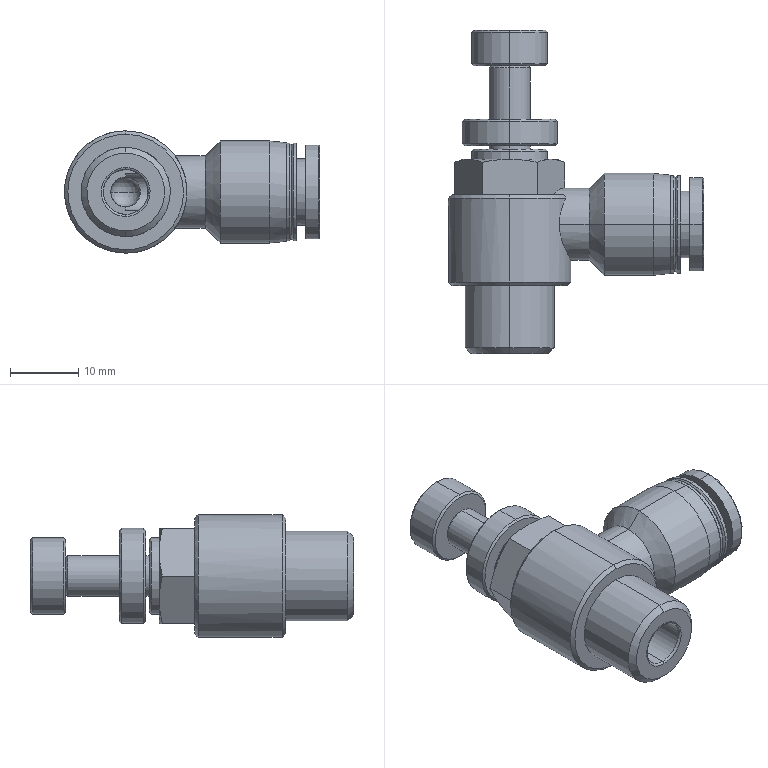Part | SolidWorks | features BaseBody 1 | 1 solid | 113 faces | box 37.5 x 47.5 x 18 mm | volume 8206 mm3 | cylinder 37 | plane 35 | cone 33 | torus 6 | sphere 2 | commonest cylinder face diameters 6 x4 11.2 x4 14.4 x4 4.386 x3 5.333 x2 6.579 x2